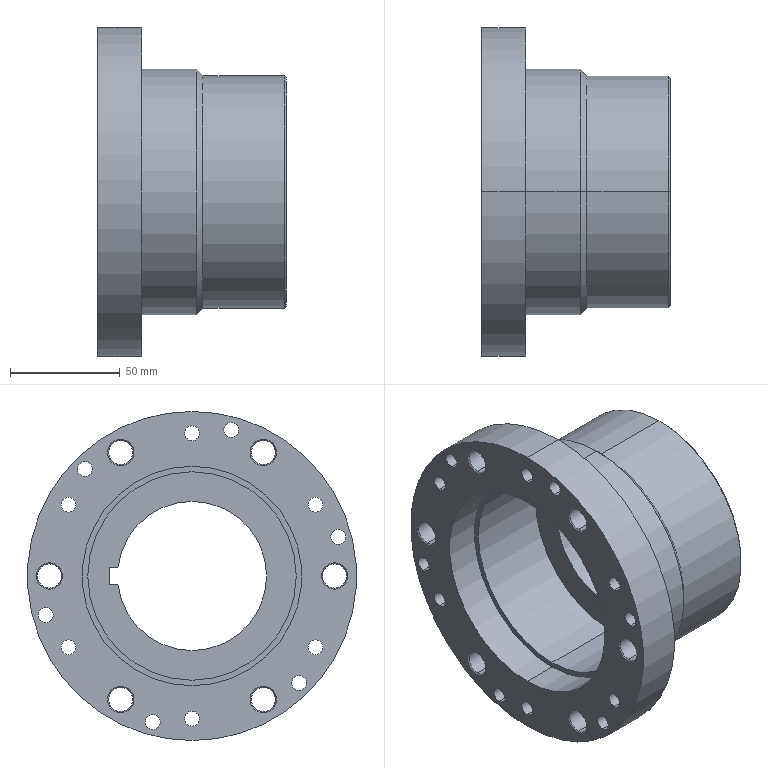Part | STEP file | 46 Belt Pulley | 1 solid | 106 faces | box 86 x 150 x 150 mm | volume 425226 mm3 | cylinder 61 | cone 31 | plane 14 | commonest cylinder face diameters 6.8 x24 11 x12 17 x12 68 x3 95 x2 100 x2